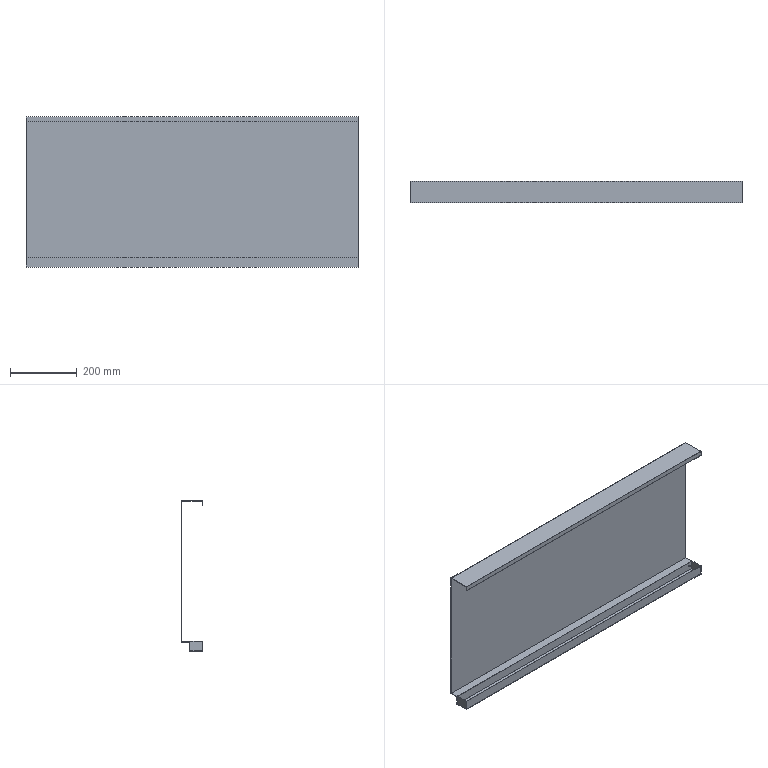Part | SolidWorks | features ICE 3, ExtruThin 1 | 3 solids | 34 faces | box 998 x 65 x 452 mm | volume 623910 mm3 | plane 30 | cylinder 4 | commonest cylinder face diameters 5.5 x4
STEP:
#1=CARTESIAN_POINT('',(0.,-26.,-401.));
#2=VERTEX_POINT('',#1);
#3=CARTESIAN_POINT('',(0.,-64.,-401.));
#4=VERTEX_POINT('',#3);
#5=CARTESIAN_POINT('',(0.,-64.,-401.));
#6=DIRECTION('',(0.,-1.,0.));
#7=VECTOR('',#6,1000.);
#8=LINE('',#5,#7);
#9=EDGE_CURVE('',#2,#4,#8,.T.);
#10=ORIENTED_EDGE('',*,*,#9,.F.);
#11=CARTESIAN_POINT('',(1.,-26.,-401.));
#12=VERTEX_POINT('',#11);
#13=CARTESIAN_POINT('',(1.,-26.,-401.));
#14=DIRECTION('',(-1.,0.,0.));
#15=VECTOR('',#14,1000.);
#16=LINE('',#13,#15);
#17=EDGE_CURVE('',#12,#2,#16,.T.);
#18=ORIENTED_EDGE('',*,*,#17,.F.);
#19=CARTESIAN_POINT('',(1.,-64.,-401.));
#20=VERTEX_POINT('',#19);
#21=CARTESIAN_POINT('',(1.,-64.,-401.));
#22=DIRECTION('',(0.,-1.,0.));
#23=VECTOR('',#22,1000.);
#24=LINE('',#21,#23);
#25=EDGE_CURVE('',#12,#20,#24,.T.);
#26=ORIENTED_EDGE('',*,*,#25,.T.);
#27=CARTESIAN_POINT('',(1.,-64.,-401.));
#28=DIRECTION('',(-1.,0.,0.));
#29=VECTOR('',#28,1000.);
#30=LINE('',#27,#29);
#31=EDGE_CURVE('',#20,#4,#30,.T.);
#32=ORIENTED_EDGE('',*,*,#31,.T.);
#33=EDGE_LOOP('',(#10,#18,#26,#32));
#34=FACE_OUTER_BOUND('',#33,.T.);
#35=CARTESIAN_POINT('',(1.,-64.,-401.));
#36=DIRECTION('',(0.,0.,-1.));
#37=DIRECTION('',(0.,1.,0.));
#38=AXIS2_PLACEMENT_3D('',#35,#36,#37);
#39=PLANE('',#38);
#40=ADVANCED_FACE('',(#34),#39,.T.);
#41=CARTESIAN_POINT('',(0.,-26.,-372.));
#42=VERTEX_POINT('',#41);
#43=CARTESIAN_POINT('',(0.,-26.,-401.));
#44=DIRECTION('',(0.,0.,-1.));
#45=VECTOR('',#44,1000.);
#46=LINE('',#43,#45);
#47=EDGE_CURVE('',#42,#2,#46,.T.);
#48=ORIENTED_EDGE('',*,*,#47,.F.);
#49=CARTESIAN_POINT('',(1.,-26.,-372.));
#50=VERTEX_POINT('',#49);
#51=CARTESIAN_POINT('',(1.,-26.,-372.));
#52=DIRECTION('',(-1.,0.,0.));
#53=VECTOR('',#52,1000.);
#54=LINE('',#51,#53);
#55=EDGE_CURVE('',#50,#42,#54,.T.);
#56=ORIENTED_EDGE('',*,*,#55,.F.);
#57=CARTESIAN_POINT('',(1.,-26.,-401.));
#58=DIRECTION('',(0.,0.,-1.));
#59=VECTOR('',#58,1000.);
#60=LINE('',#57,#59);
#61=EDGE_CURVE('',#50,#12,#60,.T.);
#62=ORIENTED_EDGE('',*,*,#61,.T.);
#63=ORIENTED_EDGE('',*,*,#17,.T.);
#64=EDGE_LOOP('',(#48,#56,#62,#63));
#65=FACE_OUTER_BOUND('',#64,.T.);
#66=CARTESIAN_POINT('',(1.,-26.,-401.));
#67=DIRECTION('',(0.,1.,0.));
#68=DIRECTION('',(0.,0.,1.));
#69=AXIS2_PLACEMENT_3D('',#66,#67,#68);
#70=PLANE('',#69);
#71=ADVANCED_FACE('',(#65),#70,.T.);
#72=CARTESIAN_POINT('',(0.,-64.,-372.));
#73=VERTEX_POINT('',#72);
#74=CARTESIAN_POINT('',(0.,-26.,-372.));
#75=DIRECTION('',(0.,1.,0.));
#76=VECTOR('',#75,1000.);
#77=LINE('',#74,#76);
#78=EDGE_CURVE('',#73,#42,#77,.T.);
#79=ORIENTED_EDGE('',*,*,#78,.F.);
#80=CARTESIAN_POINT('',(1.,-64.,-372.));
#81=VERTEX_POINT('',#80);
#82=CARTESIAN_POINT('',(1.,-64.,-372.));
#83=DIRECTION('',(-1.,0.,0.));
#84=VECTOR('',#83,1000.);
#85=LINE('',#82,#84);
#86=EDGE_CURVE('',#81,#73,#85,.T.);
#87=ORIENTED_EDGE('',*,*,#86,.F.);
#88=CARTESIAN_POINT('',(1.,-26.,-372.));
#89=DIRECTION('',(0.,1.,0.));
#90=VECTOR('',#89,1000.);
#91=LINE('',#88,#90);
#92=EDGE_CURVE('',#81,#50,#91,.T.);
#93=ORIENTED_EDGE('',*,*,#92,.T.);
#94=ORIENTED_EDGE('',*,*,#55,.T.);
#95=EDGE_LOOP('',(#79,#87,#93,#94));
#96=FACE_OUTER_BOUND('',#95,.T.);
#97=CARTESIAN_POINT('',(1.,-26.,-372.));
#98=DIRECTION('',(0.,0.,1.));
#99=DIRECTION('',(1.,0.,0.));
#100=AXIS2_PLACEMENT_3D('',#97,#98,#99);
#101=PLANE('',#100);
#102=ADVANCED_FACE('',(#96),#101,.T.);
#103=CARTESIAN_POINT('',(0.,-64.,-372.));
#104=DIRECTION('',(0.,0.,1.));
#105=VECTOR('',#104,1000.);
#106=LINE('',#103,#105);
#107=EDGE_CURVE('',#4,#73,#106,.T.);
#108=ORIENTED_EDGE('',*,*,#107,.F.);
#109=ORIENTED_EDGE('',*,*,#31,.F.);
#110=CARTESIAN_POINT('',(1.,-64.,-372.));
#111=DIRECTION('',(0.,0.,1.));
#112=VECTOR('',#111,1000.);
#113=LINE('',#110,#112);
#114=EDGE_CURVE('',#20,#81,#113,.T.);
#115=ORIENTED_EDGE('',*,*,#114,.T.);
#116=ORIENTED_EDGE('',*,*,#86,.T.);
#117=EDGE_LOOP('',(#108,#109,#115,#116));
#118=FACE_OUTER_BOUND('',#117,.T.);
#119=CARTESIAN_POINT('',(1.,-64.,-372.));
#120=DIRECTION('',(0.,-1.,0.));
#121=DIRECTION('',(0.,0.,-1.));
#122=AXIS2_PLACEMENT_3D('',#119,#120,#121);
#123=PLANE('',#122);
#124=ADVANCED_FACE('',(#118),#123,.T.);
#125=ORIENTED_EDGE('',*,*,#25,.F.);
#126=ORIENTED_EDGE('',*,*,#61,.F.);
#127=ORIENTED_EDGE('',*,*,#92,.F.);
#128=ORIENTED_EDGE('',*,*,#114,.F.);
#129=EDGE_LOOP('',(#125,#126,#127,#128));
#130=FACE_OUTER_BOUND('',#129,.T.);
#131=CARTESIAN_POINT('',(1.,-26.,-401.));
#132=DIRECTION('',(1.,0.,0.));
#133=DIRECTION('',(0.,0.,-1.));
#134=AXIS2_PLACEMENT_3D('',#131,#132,#133);
#135=PLANE('',#134);
#136=ADVANCED_FACE('',(#130),#135,.T.);
#137=ORIENTED_EDGE('',*,*,#9,.T.);
#138=ORIENTED_EDGE('',*,*,#107,.T.);
#139=ORIENTED_EDGE('',*,*,#78,.T.);
#140=ORIENTED_EDGE('',*,*,#47,.T.);
#141=EDGE_LOOP('',(#137,#138,#139,#140));
#142=FACE_OUTER_BOUND('',#141,.T.);
#143=CARTESIAN_POINT('',(0.,-26.,-401.));
#144=DIRECTION('',(1.,0.,0.));
#145=DIRECTION('',(0.,0.,-1.));
#146=AXIS2_PLACEMENT_3D('',#143,#144,#145);
#147=PLANE('',#146);
#148=ADVANCED_FACE('',(#142),#147,.F.);
#149=CLOSED_SHELL('',(#40,#71,#102,#124,#136,#148));
#150=MANIFOLD_SOLID_BREP('',#149);
#151=CARTESIAN_POINT('',(998.,-26.,-372.));
#152=VERTEX_POINT('',#151);
#153=CARTESIAN_POINT('',(998.,-64.,-372.));
#154=VERTEX_POINT('',#153);
#155=CARTESIAN_POINT('',(998.,-26.,-372.));
#156=DIRECTION('',(0.,-1.,0.));
#157=VECTOR('',#156,1000.);
#158=LINE('',#155,#157);
#159=EDGE_CURVE('',#152,#154,#158,.T.);
#160=ORIENTED_EDGE('',*,*,#159,.F.);
#161=CARTESIAN_POINT('',(997.,-26.,-372.));
#162=VERTEX_POINT('',#161);
#163=CARTESIAN_POINT('',(997.,-26.,-372.));
#164=DIRECTION('',(1.,0.,0.));
#165=VECTOR('',#164,1000.);
#166=LINE('',#163,#165);
#167=EDGE_CURVE('',#162,#152,#166,.T.);
#168=ORIENTED_EDGE('',*,*,#167,.F.);
#169=CARTESIAN_POINT('',(997.,-64.,-372.));
#170=VERTEX_POINT('',#169);
#171=CARTESIAN_POINT('',(997.,-26.,-372.));
#172=DIRECTION('',(0.,-1.,0.));
#173=VECTOR('',#172,1000.);
#174=LINE('',#171,#173);
#175=EDGE_CURVE('',#162,#170,#174,.T.);
#176=ORIENTED_EDGE('',*,*,#175,.T.);
#177=CARTESIAN_POINT('',(997.,-64.,-372.));
#178=DIRECTION('',(1.,0.,0.));
#179=VECTOR('',#178,1000.);
#180=LINE('',#177,#179);
#181=EDGE_CURVE('',#170,#154,#180,.T.);
#182=ORIENTED_EDGE('',*,*,#181,.T.);
#183=EDGE_LOOP('',(#160,#168,#176,#182));
#184=FACE_OUTER_BOUND('',#183,.T.);
#185=CARTESIAN_POINT('',(997.,-26.,-372.));
#186=DIRECTION('',(0.,0.,1.));
#187=DIRECTION('',(1.,0.,0.));
#188=AXIS2_PLACEMENT_3D('',#185,#186,#187);
#189=PLANE('',#188);
#190=ADVANCED_FACE('',(#184),#189,.T.);
#191=CARTESIAN_POINT('',(998.,-26.,-401.));
#192=VERTEX_POINT('',#191);
#193=CARTESIAN_POINT('',(998.,-26.,-401.));
#194=DIRECTION('',(0.,0.,1.));
#195=VECTOR('',#194,1000.);
#196=LINE('',#193,#195);
#197=EDGE_CURVE('',#192,#152,#196,.T.);
#198=ORIENTED_EDGE('',*,*,#197,.F.);
#199=CARTESIAN_POINT('',(997.,-26.,-401.));
#200=VERTEX_POINT('',#199);
#201=CARTESIAN_POINT('',(997.,-26.,-401.));
#202=DIRECTION('',(1.,0.,0.));
#203=VECTOR('',#202,1000.);
#204=LINE('',#201,#203);
#205=EDGE_CURVE('',#200,#192,#204,.T.);
#206=ORIENTED_EDGE('',*,*,#205,.F.);
#207=CARTESIAN_POINT('',(997.,-26.,-401.));
#208=DIRECTION('',(0.,0.,1.));
#209=VECTOR('',#208,1000.);
#210=LINE('',#207,#209);
#211=EDGE_CURVE('',#200,#162,#210,.T.);
#212=ORIENTED_EDGE('',*,*,#211,.T.);
#213=ORIENTED_EDGE('',*,*,#167,.T.);
#214=EDGE_LOOP('',(#198,#206,#212,#213));
#215=FACE_OUTER_BOUND('',#214,.T.);
#216=CARTESIAN_POINT('',(997.,-26.,-401.));
#217=DIRECTION('',(0.,1.,0.));
#218=DIRECTION('',(0.,0.,1.));
#219=AXIS2_PLACEMENT_3D('',#216,#217,#218);
#220=PLANE('',#219);
#221=ADVANCED_FACE('',(#215),#220,.T.);
#222=CARTESIAN_POINT('',(998.,-64.,-401.));
#223=VERTEX_POINT('',#222);
#224=CARTESIAN_POINT('',(998.,-64.,-401.));
#225=DIRECTION('',(0.,1.,0.));
#226=VECTOR('',#225,1000.);
#227=LINE('',#224,#226);
#228=EDGE_CURVE('',#223,#192,#227,.T.);
#229=ORIENTED_EDGE('',*,*,#228,.F.);
#230=CARTESIAN_POINT('',(997.,-64.,-401.));
#231=VERTEX_POINT('',#230);
#232=CARTESIAN_POINT('',(997.,-64.,-401.));
#233=DIRECTION('',(1.,0.,0.));
#234=VECTOR('',#233,1000.);
#235=LINE('',#232,#234);
#236=EDGE_CURVE('',#231,#223,#235,.T.);
#237=ORIENTED_EDGE('',*,*,#236,.F.);
#238=CARTESIAN_POINT('',(997.,-64.,-401.));
#239=DIRECTION('',(0.,1.,0.));
#240=VECTOR('',#239,1000.);
#241=LINE('',#238,#240);
#242=EDGE_CURVE('',#231,#200,#241,.T.);
#243=ORIENTED_EDGE('',*,*,#242,.T.);
#244=ORIENTED_EDGE('',*,*,#205,.T.);
#245=EDGE_LOOP('',(#229,#237,#243,#244));
#246=FACE_OUTER_BOUND('',#245,.T.);
#247=CARTESIAN_POINT('',(997.,-64.,-401.));
#248=DIRECTION('',(0.,0.,-1.));
#249=DIRECTION('',(0.,1.,0.));
#250=AXIS2_PLACEMENT_3D('',#247,#248,#249);
#251=PLANE('',#250);
#252=ADVANCED_FACE('',(#246),#251,.T.);
#253=CARTESIAN_POINT('',(998.,-64.,-372.));
#254=DIRECTION('',(0.,0.,-1.));
#255=VECTOR('',#254,1000.);
#256=LINE('',#253,#255);
#257=EDGE_CURVE('',#154,#223,#256,.T.);
#258=ORIENTED_EDGE('',*,*,#257,.F.);
#259=ORIENTED_EDGE('',*,*,#181,.F.);
#260=CARTESIAN_POINT('',(997.,-64.,-372.));
#261=DIRECTION('',(0.,0.,-1.));
#262=VECTOR('',#261,1000.);
#263=LINE('',#260,#262);
#264=EDGE_CURVE('',#170,#231,#263,.T.);
#265=ORIENTED_EDGE('',*,*,#264,.T.);
#266=ORIENTED_EDGE('',*,*,#236,.T.);
#267=EDGE_LOOP('',(#258,#259,#265,#266));
#268=FACE_OUTER_BOUND('',#267,.T.);
#269=CARTESIAN_POINT('',(997.,-64.,-372.));
#270=DIRECTION('',(0.,-1.,0.));
#271=DIRECTION('',(0.,0.,-1.));
#272=AXIS2_PLACEMENT_3D('',#269,#270,#271);
#273=PLANE('',#272);
#274=ADVANCED_FACE('',(#268),#273,.T.);
#275=ORIENTED_EDGE('',*,*,#175,.F.);
#276=ORIENTED_EDGE('',*,*,#211,.F.);
#277=ORIENTED_EDGE('',*,*,#242,.F.);
#278=ORIENTED_EDGE('',*,*,#264,.F.);
#279=EDGE_LOOP('',(#275,#276,#277,#278));
#280=FACE_OUTER_BOUND('',#279,.T.);
#281=CARTESIAN_POINT('',(997.,-64.,-372.));
#282=DIRECTION('',(1.,0.,0.));
#283=DIRECTION('',(0.,0.,-1.));
#284=AXIS2_PLACEMENT_3D('',#281,#282,#283);
#285=PLANE('',#284);
#286=ADVANCED_FACE('',(#280),#285,.F.);
#287=ORIENTED_EDGE('',*,*,#159,.T.);
#288=ORIENTED_EDGE('',*,*,#257,.T.);
#289=ORIENTED_EDGE('',*,*,#228,.T.);
#290=ORIENTED_EDGE('',*,*,#197,.T.);
#291=EDGE_LOOP('',(#287,#288,#289,#290));
#292=FACE_OUTER_BOUND('',#291,.T.);
#293=CARTESIAN_POINT('',(998.,-64.,-372.));
#294=DIRECTION('',(1.,0.,0.));
#295=DIRECTION('',(0.,0.,-1.));
#296=AXIS2_PLACEMENT_3D('',#293,#294,#295);
#297=PLANE('',#296);
#298=ADVANCED_FACE('',(#292),#297,.T.);
#299=CLOSED_SHELL('',(#190,#221,#252,#274,#286,#298));
#300=MANIFOLD_SOLID_BREP('',#299);
#301=CARTESIAN_POINT('',(988.,-26.,-384.25));
#302=VERTEX_POINT('',#301);
#303=CARTESIAN_POINT('',(988.,-26.,-389.75));
#304=VERTEX_POINT('',#303);
#305=CARTESIAN_POINT('',(988.,-26.,-387.));
#306=DIRECTION('',(0.,-1.,0.));
#307=DIRECTION('',(0.,0.,-1.));
#308=AXIS2_PLACEMENT_3D('',#305,#306,#307);
#309=CIRCLE('',#308,2.75);
#310=EDGE_CURVE('',#302,#304,#309,.T.);
#311=ORIENTED_EDGE('',*,*,#310,.T.);
#312=CARTESIAN_POINT('',(988.,-25.,-389.75));
#313=VERTEX_POINT('',#312);
#314=CARTESIAN_POINT('',(988.,-35.,-389.75));
#315=DIRECTION('',(0.,1.,0.));
#316=VECTOR('',#315,1000.);
#317=LINE('',#314,#316);
#318=EDGE_CURVE('',#304,#313,#317,.T.);
#319=ORIENTED_EDGE('',*,*,#318,.T.);
#320=CARTESIAN_POINT('',(988.,-25.,-384.25));
#321=VERTEX_POINT('',#320);
#322=CARTESIAN_POINT('',(988.,-25.,-387.));
#323=DIRECTION('',(0.,1.,0.));
#324=DIRECTION('',(0.,0.,1.));
#325=AXIS2_PLACEMENT_3D('',#322,#323,#324);
#326=CIRCLE('',#325,2.75);
#327=EDGE_CURVE('',#313,#321,#326,.T.);
#328=ORIENTED_EDGE('',*,*,#327,.T.);
#329=CARTESIAN_POINT('',(988.,-35.,-384.25));
#330=DIRECTION('',(0.,1.,0.));
#331=VECTOR('',#330,1000.);
#332=LINE('',#329,#331);
#333=EDGE_CURVE('',#302,#321,#332,.T.);
#334=ORIENTED_EDGE('',*,*,#333,.F.);
#335=EDGE_LOOP('',(#311,#319,#328,#334));
#336=FACE_OUTER_BOUND('',#335,.T.);
#337=CARTESIAN_POINT('',(988.,-35.,-387.));
#338=DIRECTION('',(0.,1.,0.));
#339=DIRECTION('',(0.,0.,1.));
#340=AXIS2_PLACEMENT_3D('',#337,#338,#339);
#341=CYLINDRICAL_SURFACE('',#340,2.75);
#342=ADVANCED_FACE('',(#336),#341,.F.);
#343=CARTESIAN_POINT('',(13.,-26.,-386.25));
#344=VERTEX_POINT('',#343);
#345=CARTESIAN_POINT('',(13.,-26.,-391.75));
#346=VERTEX_POINT('',#345);
#347=CARTESIAN_POINT('',(13.,-26.,-389.));
#348=DIRECTION('',(0.,-1.,0.));
#349=DIRECTION('',(0.,0.,-1.));
#350=AXIS2_PLACEMENT_3D('',#347,#348,#349);
#351=CIRCLE('',#350,2.75);
#352=EDGE_CURVE('',#344,#346,#351,.T.);
#353=ORIENTED_EDGE('',*,*,#352,.T.);
#354=CARTESIAN_POINT('',(13.,-25.,-391.75));
#355=VERTEX_POINT('',#354);
#356=CARTESIAN_POINT('',(13.,-35.,-391.75));
#357=DIRECTION('',(0.,1.,0.));
#358=VECTOR('',#357,1000.);
#359=LINE('',#356,#358);
#360=EDGE_CURVE('',#346,#355,#359,.T.);
#361=ORIENTED_EDGE('',*,*,#360,.T.);
#362=CARTESIAN_POINT('',(13.,-25.,-386.25));
#363=VERTEX_POINT('',#362);
#364=CARTESIAN_POINT('',(13.,-25.,-389.));
#365=DIRECTION('',(0.,1.,0.));
#366=DIRECTION('',(0.,0.,1.));
#367=AXIS2_PLACEMENT_3D('',#364,#365,#366);
#368=CIRCLE('',#367,2.75);
#369=EDGE_CURVE('',#355,#363,#368,.T.);
#370=ORIENTED_EDGE('',*,*,#369,.T.);
#371=CARTESIAN_POINT('',(13.,-35.,-386.25));
#372=DIRECTION('',(0.,1.,0.));
#373=VECTOR('',#372,1000.);
#374=LINE('',#371,#373);
#375=EDGE_CURVE('',#344,#363,#374,.T.);
#376=ORIENTED_EDGE('',*,*,#375,.F.);
#377=EDGE_LOOP('',(#353,#361,#370,#376));
#378=FACE_OUTER_BOUND('',#377,.T.);
#379=CARTESIAN_POINT('',(13.,-35.,-389.));
#380=DIRECTION('',(0.,1.,0.));
#381=DIRECTION('',(0.,0.,1.));
#382=AXIS2_PLACEMENT_3D('',#379,#380,#381);
#383=CYLINDRICAL_SURFACE('',#382,2.75);
#384=ADVANCED_FACE('',(#378),#383,.F.);
#385=CARTESIAN_POINT('',(0.,-65.,50.));
#386=VERTEX_POINT('',#385);
#387=CARTESIAN_POINT('',(0.,-65.,35.));
#388=VERTEX_POINT('',#387);
#389=CARTESIAN_POINT('',(0.,-65.,50.));
#390=DIRECTION('',(0.,0.,-1.));
#391=VECTOR('',#390,1000.);
#392=LINE('',#389,#391);
#393=EDGE_CURVE('',#386,#388,#392,.T.);
#394=ORIENTED_EDGE('',*,*,#393,.T.);
#395=CARTESIAN_POINT('',(998.,-65.,35.));
#396=VERTEX_POINT('',#395);
#397=CARTESIAN_POINT('',(998.,-65.,35.));
#398=DIRECTION('',(-1.,0.,0.));
#399=VECTOR('',#398,1000.);
#400=LINE('',#397,#399);
#401=EDGE_CURVE('',#396,#388,#400,.T.);
#402=ORIENTED_EDGE('',*,*,#401,.F.);
#403=CARTESIAN_POINT('',(998.,-65.,50.));
#404=VERTEX_POINT('',#403);
#405=CARTESIAN_POINT('',(998.,-65.,50.));
#406=DIRECTION('',(0.,0.,-1.));
#407=VECTOR('',#406,1000.);
#408=LINE('',#405,#407);
#409=EDGE_CURVE('',#404,#396,#408,.T.);
#410=ORIENTED_EDGE('',*,*,#409,.F.);
#411=CARTESIAN_POINT('',(998.,-65.,50.));
#412=DIRECTION('',(-1.,0.,0.));
#413=VECTOR('',#412,1000.);
#414=LINE('',#411,#413);
#415=EDGE_CURVE('',#404,#386,#414,.T.);
#416=ORIENTED_EDGE('',*,*,#415,.T.);
#417=EDGE_LOOP('',(#394,#402,#410,#416));
#418=FACE_OUTER_BOUND('',#417,.T.);
#419=CARTESIAN_POINT('',(998.,-65.,50.));
#420=DIRECTION('',(0.,1.,0.));
#421=DIRECTION('',(0.,0.,1.));
#422=AXIS2_PLACEMENT_3D('',#419,#420,#421);
#423=PLANE('',#422);
#424=ADVANCED_FACE('',(#418),#423,.F.);
#425=CARTESIAN_POINT('',(0.,-64.,35.));
#426=VERTEX_POINT('',#425);
#427=CARTESIAN_POINT('',(0.,-64.,35.));
#428=DIRECTION('',(0.,-1.,0.));
#429=VECTOR('',#428,1000.);
#430=LINE('',#427,#429);
#431=EDGE_CURVE('',#426,#388,#430,.T.);
#432=ORIENTED_EDGE('',*,*,#431,.F.);
#433=CARTESIAN_POINT('',(998.,-64.,35.));
#434=VERTEX_POINT('',#433);
#435=CARTESIAN_POINT('',(998.,-64.,35.));
#436=DIRECTION('',(-1.,0.,0.));
#437=VECTOR('',#436,1000.);
#438=LINE('',#435,#437);
#439=EDGE_CURVE('',#434,#426,#438,.T.);
#440=ORIENTED_EDGE('',*,*,#439,.F.);
#441=CARTESIAN_POINT('',(998.,-64.,35.));
#442=DIRECTION('',(0.,-1.,0.));
#443=VECTOR('',#442,1000.);
#444=LINE('',#441,#443);
#445=EDGE_CURVE('',#434,#396,#444,.T.);
#446=ORIENTED_EDGE('',*,*,#445,.T.);
#447=ORIENTED_EDGE('',*,*,#401,.T.);
#448=EDGE_LOOP('',(#432,#440,#446,#447));
#449=FACE_OUTER_BOUND('',#448,.T.);
#450=CARTESIAN_POINT('',(998.,-64.,35.));
#451=DIRECTION('',(0.,0.,-1.));
#452=DIRECTION('',(-1.,0.,0.));
#453=AXIS2_PLACEMENT_3D('',#450,#451,#452);
#454=PLANE('',#453);
#455=ADVANCED_FACE('',(#449),#454,.T.);
#456=CARTESIAN_POINT('',(0.,-64.,49.));
#457=VERTEX_POINT('',#456);
#458=CARTESIAN_POINT('',(0.,-64.,50.));
#459=DIRECTION('',(0.,0.,-1.));
#460=VECTOR('',#459,1000.);
#461=LINE('',#458,#460);
#462=EDGE_CURVE('',#457,#426,#461,.T.);
#463=ORIENTED_EDGE('',*,*,#462,.F.);
#464=CARTESIAN_POINT('',(998.,-64.,49.));
#465=VERTEX_POINT('',#464);
#466=CARTESIAN_POINT('',(998.,-64.,49.));
#467=DIRECTION('',(-1.,0.,0.));
#468=VECTOR('',#467,1000.);
#469=LINE('',#466,#468);
#470=EDGE_CURVE('',#465,#457,#469,.T.);
#471=ORIENTED_EDGE('',*,*,#470,.F.);
#472=CARTESIAN_POINT('',(998.,-64.,50.));
#473=DIRECTION('',(0.,0.,-1.));
#474=VECTOR('',#473,1000.);
#475=LINE('',#472,#474);
#476=EDGE_CURVE('',#465,#434,#475,.T.);
#477=ORIENTED_EDGE('',*,*,#476,.T.);
#478=ORIENTED_EDGE('',*,*,#439,.T.);
#479=EDGE_LOOP('',(#463,#471,#477,#478));
#480=FACE_OUTER_BOUND('',#479,.T.);
#481=CARTESIAN_POINT('',(998.,-64.,50.));
#482=DIRECTION('',(0.,1.,0.));
#483=DIRECTION('',(0.,0.,1.));
#484=AXIS2_PLACEMENT_3D('',#481,#482,#483);
#485=PLANE('',#484);
#486=ADVANCED_FACE('',(#480),#485,.T.);
#487=CARTESIAN_POINT('',(0.,-1.,49.));
#488=VERTEX_POINT('',#487);
#489=CARTESIAN_POINT('',(0.,0.,49.));
#490=DIRECTION('',(0.,-1.,0.));
#491=VECTOR('',#490,1000.);
#492=LINE('',#489,#491);
#493=EDGE_CURVE('',#488,#457,#492,.T.);
#494=ORIENTED_EDGE('',*,*,#493,.F.);
#495=CARTESIAN_POINT('',(998.,-1.,49.));
#496=VERTEX_POINT('',#495);
#497=CARTESIAN_POINT('',(998.,-1.,49.));
#498=DIRECTION('',(-1.,0.,0.));
#499=VECTOR('',#498,1000.);
#500=LINE('',#497,#499);
#501=EDGE_CURVE('',#496,#488,#500,.T.);
#502=ORIENTED_EDGE('',*,*,#501,.F.);
#503=CARTESIAN_POINT('',(998.,0.,49.));
#504=DIRECTION('',(0.,-1.,0.));
#505=VECTOR('',#504,1000.);
#506=LINE('',#503,#505);
#507=EDGE_CURVE('',#496,#465,#506,.T.);
#508=ORIENTED_EDGE('',*,*,#507,.T.);
#509=ORIENTED_EDGE('',*,*,#470,.T.);
#510=EDGE_LOOP('',(#494,#502,#508,#509));
#511=FACE_OUTER_BOUND('',#510,.T.);
#512=CARTESIAN_POINT('',(998.,0.,49.));
#513=DIRECTION('',(0.,0.,-1.));
#514=DIRECTION('',(0.,1.,0.));
#515=AXIS2_PLACEMENT_3D('',#512,#513,#514);
#516=PLANE('',#515);
#517=ADVANCED_FACE('',(#511),#516,.T.);
#518=CARTESIAN_POINT('',(0.,-1.,-374.));
#519=VERTEX_POINT('',#518);
#520=CARTESIAN_POINT('',(0.,-1.,0.));
#521=DIRECTION('',(0.,0.,1.));
#522=VECTOR('',#521,1000.);
#523=LINE('',#520,#522);
#524=EDGE_CURVE('',#519,#488,#523,.T.);
#525=ORIENTED_EDGE('',*,*,#524,.F.);
#526=CARTESIAN_POINT('',(998.,-1.,-374.));
#527=VERTEX_POINT('',#526);
#528=CARTESIAN_POINT('',(998.,-1.,-374.));
#529=DIRECTION('',(-1.,0.,0.));
#530=VECTOR('',#529,1000.);
#531=LINE('',#528,#530);
#532=EDGE_CURVE('',#527,#519,#531,.T.);
#533=ORIENTED_EDGE('',*,*,#532,.F.);
#534=CARTESIAN_POINT('',(998.,-1.,0.));
#535=DIRECTION('',(0.,0.,1.));
#536=VECTOR('',#535,1000.);
#537=LINE('',#534,#536);
#538=EDGE_CURVE('',#527,#496,#537,.T.);
#539=ORIENTED_EDGE('',*,*,#538,.T.);
#540=ORIENTED_EDGE('',*,*,#501,.T.);
#541=EDGE_LOOP('',(#525,#533,#539,#540));
#542=FACE_OUTER_BOUND('',#541,.T.);
#543=CARTESIAN_POINT('',(998.,-1.,0.));
#544=DIRECTION('',(0.,-1.,0.));
#545=DIRECTION('',(0.,0.,-1.));
#546=AXIS2_PLACEMENT_3D('',#543,#544,#545);
#547=PLANE('',#546);
#548=ADVANCED_FACE('',(#542),#547,.T.);
#549=CARTESIAN_POINT('',(0.,-26.,-374.));
#550=VERTEX_POINT('',#549);
#551=CARTESIAN_POINT('',(0.,0.,-374.));
#552=DIRECTION('',(0.,1.,0.));
#553=VECTOR('',#552,1000.);
#554=LINE('',#551,#553);
#555=EDGE_CURVE('',#550,#519,#554,.T.);
#556=ORIENTED_EDGE('',*,*,#555,.F.);
#557=CARTESIAN_POINT('',(998.,-26.,-374.));
#558=VERTEX_POINT('',#557);
#559=CARTESIAN_POINT('',(998.,-26.,-374.));
#560=DIRECTION('',(-1.,0.,0.));
#561=VECTOR('',#560,1000.);
#562=LINE('',#559,#561);
#563=EDGE_CURVE('',#558,#550,#562,.T.);
#564=ORIENTED_EDGE('',*,*,#563,.F.);
#565=CARTESIAN_POINT('',(998.,0.,-374.));
#566=DIRECTION('',(0.,1.,0.));
#567=VECTOR('',#566,1000.);
#568=LINE('',#565,#567);
#569=EDGE_CURVE('',#558,#527,#568,.T.);
#570=ORIENTED_EDGE('',*,*,#569,.T.);
#571=ORIENTED_EDGE('',*,*,#532,.T.);
#572=EDGE_LOOP('',(#556,#564,#570,#571));
#573=FACE_OUTER_BOUND('',#572,.T.);
#574=CARTESIAN_POINT('',(998.,0.,-374.));
#575=DIRECTION('',(0.,0.,1.));
#576=DIRECTION('',(1.,0.,0.));
#577=AXIS2_PLACEMENT_3D('',#574,#575,#576);
#578=PLANE('',#577);
#579=ADVANCED_FACE('',(#573),#578,.T.);
#580=ORIENTED_EDGE('',*,*,#310,.F.);
#581=CARTESIAN_POINT('',(988.,-26.,-387.));
#582=DIRECTION('',(0.,-1.,0.));
#583=DIRECTION('',(0.,0.,-1.));
#584=AXIS2_PLACEMENT_3D('',#581,#582,#583);
#585=CIRCLE('',#584,2.75);
#586=EDGE_CURVE('',#304,#302,#585,.T.);
#587=ORIENTED_EDGE('',*,*,#586,.F.);
#588=EDGE_LOOP('',(#580,#587));
#589=FACE_BOUND('',#588,.T.);
#590=ORIENTED_EDGE('',*,*,#352,.F.);
#591=CARTESIAN_POINT('',(13.,-26.,-389.));
#592=DIRECTION('',(0.,-1.,0.));
#593=DIRECTION('',(0.,0.,-1.));
#594=AXIS2_PLACEMENT_3D('',#591,#592,#593);
#595=CIRCLE('',#594,2.75);
#596=EDGE_CURVE('',#346,#344,#595,.T.);
#597=ORIENTED_EDGE('',*,*,#596,.F.);
#598=EDGE_LOOP('',(#590,#597));
#599=FACE_BOUND('',#598,.T.);
#600=CARTESIAN_POINT('',(0.,-26.,-401.));
#601=VERTEX_POINT('',#600);
#602=CARTESIAN_POINT('',(0.,-26.,-375.));
#603=DIRECTION('',(0.,0.,1.));
#604=VECTOR('',#603,1000.);
#605=LINE('',#602,#604);
#606=EDGE_CURVE('',#601,#550,#605,.T.);
#607=ORIENTED_EDGE('',*,*,#606,.F.);
#608=CARTESIAN_POINT('',(998.,-26.,-401.));
#609=VERTEX_POINT('',#608);
#610=CARTESIAN_POINT('',(998.,-26.,-401.));
#611=DIRECTION('',(-1.,0.,0.));
#612=VECTOR('',#611,1000.);
#613=LINE('',#610,#612);
#614=EDGE_CURVE('',#609,#601,#613,.T.);
#615=ORIENTED_EDGE('',*,*,#614,.F.);
#616=CARTESIAN_POINT('',(998.,-26.,-375.));
#617=DIRECTION('',(0.,0.,1.));
#618=VECTOR('',#617,1000.);
#619=LINE('',#616,#618);
#620=EDGE_CURVE('',#609,#558,#619,.T.);
#621=ORIENTED_EDGE('',*,*,#620,.T.);
#622=ORIENTED_EDGE('',*,*,#563,.T.);
#623=EDGE_LOOP('',(#607,#615,#621,#622));
#624=FACE_OUTER_BOUND('',#623,.T.);
#625=CARTESIAN_POINT('',(998.,-26.,-375.));
#626=DIRECTION('',(0.,-1.,0.));
#627=DIRECTION('',(0.,0.,-1.));
#628=AXIS2_PLACEMENT_3D('',#625,#626,#627);
#629=PLANE('',#628);
#630=ADVANCED_FACE('',(#589,#599,#624),#629,.T.);
#631=CARTESIAN_POINT('',(0.,-64.,-401.));
#632=VERTEX_POINT('',#631);
#633=CARTESIAN_POINT('',(0.,-25.,-401.));
#634=DIRECTION('',(0.,1.,0.));
#635=VECTOR('',#634,1000.);
#636=LINE('',#633,#635);
#637=EDGE_CURVE('',#632,#601,#636,.T.);
#638=ORIENTED_EDGE('',*,*,#637,.F.);
#639=CARTESIAN_POINT('',(998.,-64.,-401.));
#640=VERTEX_POINT('',#639);
#641=CARTESIAN_POINT('',(998.,-64.,-401.));
#642=DIRECTION('',(-1.,0.,0.));
#643=VECTOR('',#642,1000.);
#644=LINE('',#641,#643);
#645=EDGE_CURVE('',#640,#632,#644,.T.);
#646=ORIENTED_EDGE('',*,*,#645,.F.);
#647=CARTESIAN_POINT('',(998.,-25.,-401.));
#648=DIRECTION('',(0.,1.,0.));
#649=VECTOR('',#648,1000.);
#650=LINE('',#647,#649);
#651=EDGE_CURVE('',#640,#609,#650,.T.);
#652=ORIENTED_EDGE('',*,*,#651,.T.);
#653=ORIENTED_EDGE('',*,*,#614,.T.);
#654=EDGE_LOOP('',(#638,#646,#652,#653));
#655=FACE_OUTER_BOUND('',#654,.T.);
#656=CARTESIAN_POINT('',(998.,-25.,-401.));
#657=DIRECTION('',(0.,0.,1.));
#658=DIRECTION('',(0.,-1.,0.));
#659=AXIS2_PLACEMENT_3D('',#656,#657,#658);
#660=PLANE('',#659);
#661=ADVANCED_FACE('',(#655),#660,.T.);
#662=CARTESIAN_POINT('',(0.,-64.,-372.));
#663=VERTEX_POINT('',#662);
#664=CARTESIAN_POINT('',(0.,-64.,-402.));
#665=DIRECTION('',(0.,0.,-1.));
#666=VECTOR('',#665,1000.);
#667=LINE('',#664,#666);
#668=EDGE_CURVE('',#663,#632,#667,.T.);
#669=ORIENTED_EDGE('',*,*,#668,.F.);
#670=CARTESIAN_POINT('',(998.,-64.,-372.));
#671=VERTEX_POINT('',#670);
#672=CARTESIAN_POINT('',(998.,-64.,-372.));
#673=DIRECTION('',(-1.,0.,0.));
#674=VECTOR('',#673,1000.);
#675=LINE('',#672,#674);
#676=EDGE_CURVE('',#671,#663,#675,.T.);
#677=ORIENTED_EDGE('',*,*,#676,.F.);
#678=CARTESIAN_POINT('',(998.,-64.,-402.));
#679=DIRECTION('',(0.,0.,-1.));
#680=VECTOR('',#679,1000.);
#681=LINE('',#678,#680);
#682=EDGE_CURVE('',#671,#640,#681,.T.);
#683=ORIENTED_EDGE('',*,*,#682,.T.);
#684=ORIENTED_EDGE('',*,*,#645,.T.);
#685=EDGE_LOOP('',(#669,#677,#683,#684));
#686=FACE_OUTER_BOUND('',#685,.T.);
#687=CARTESIAN_POINT('',(998.,-64.,-402.));
#688=DIRECTION('',(0.,1.,0.));
#689=DIRECTION('',(0.,0.,1.));
#690=AXIS2_PLACEMENT_3D('',#687,#688,#689);
#691=PLANE('',#690);
#692=ADVANCED_FACE('',(#686),#691,.T.);
#693=CARTESIAN_POINT('',(0.,-65.,-372.));
#694=VERTEX_POINT('',#693);
#695=CARTESIAN_POINT('',(0.,-65.,-372.));
#696=DIRECTION('',(0.,1.,0.));
#697=VECTOR('',#696,1000.);
#698=LINE('',#695,#697);
#699=EDGE_CURVE('',#694,#663,#698,.T.);
#700=ORIENTED_EDGE('',*,*,#699,.F.);
#701=CARTESIAN_POINT('',(998.,-65.,-372.));
#702=VERTEX_POINT('',#701);
#703=CARTESIAN_POINT('',(998.,-65.,-372.));
#704=DIRECTION('',(-1.,0.,0.));
#705=VECTOR('',#704,1000.);
#706=LINE('',#703,#705);
#707=EDGE_CURVE('',#702,#694,#706,.T.);
#708=ORIENTED_EDGE('',*,*,#707,.F.);
#709=CARTESIAN_POINT('',(998.,-65.,-372.));
#710=DIRECTION('',(0.,1.,0.));
#711=VECTOR('',#710,1000.);
#712=LINE('',#709,#711);
#713=EDGE_CURVE('',#702,#671,#712,.T.);
#714=ORIENTED_EDGE('',*,*,#713,.T.);
#715=ORIENTED_EDGE('',*,*,#676,.T.);
#716=EDGE_LOOP('',(#700,#708,#714,#715));
#717=FACE_OUTER_BOUND('',#716,.T.);
#718=CARTESIAN_POINT('',(998.,-65.,-372.));
#719=DIRECTION('',(0.,0.,1.));
#720=DIRECTION('',(1.,0.,0.));
#721=AXIS2_PLACEMENT_3D('',#718,#719,#720);
#722=PLANE('',#721);
#723=ADVANCED_FACE('',(#717),#722,.T.);
#724=CARTESIAN_POINT('',(0.,-65.,-402.));
#725=VERTEX_POINT('',#724);
#726=CARTESIAN_POINT('',(0.,-65.,-402.));
#727=DIRECTION('',(0.,0.,-1.));
#728=VECTOR('',#727,1000.);
#729=LINE('',#726,#728);
#730=EDGE_CURVE('',#694,#725,#729,.T.);
#731=ORIENTED_EDGE('',*,*,#730,.T.);
#732=CARTESIAN_POINT('',(998.,-65.,-402.));
#733=VERTEX_POINT('',#732);
#734=CARTESIAN_POINT('',(998.,-65.,-402.));
#735=DIRECTION('',(-1.,0.,0.));
#736=VECTOR('',#735,1000.);
#737=LINE('',#734,#736);
#738=EDGE_CURVE('',#733,#725,#737,.T.);
#739=ORIENTED_EDGE('',*,*,#738,.F.);
#740=CARTESIAN_POINT('',(998.,-65.,-402.));
#741=DIRECTION('',(0.,0.,-1.));
#742=VECTOR('',#741,1000.);
#743=LINE('',#740,#742);
#744=EDGE_CURVE('',#702,#733,#743,.T.);
#745=ORIENTED_EDGE('',*,*,#744,.F.);
#746=ORIENTED_EDGE('',*,*,#707,.T.);
#747=EDGE_LOOP('',(#731,#739,#745,#746));
#748=FACE_OUTER_BOUND('',#747,.T.);
#749=CARTESIAN_POINT('',(998.,-65.,-402.));
#750=DIRECTION('',(0.,1.,0.));
#751=DIRECTION('',(0.,0.,1.));
#752=AXIS2_PLACEMENT_3D('',#749,#750,#751);
#753=PLANE('',#752);
#754=ADVANCED_FACE('',(#748),#753,.F.);
#755=CARTESIAN_POINT('',(0.,-25.,-402.));
#756=VERTEX_POINT('',#755);
#757=CARTESIAN_POINT('',(0.,-25.,-402.));
#758=DIRECTION('',(0.,1.,0.));
#759=VECTOR('',#758,1000.);
#760=LINE('',#757,#759);
#761=EDGE_CURVE('',#725,#756,#760,.T.);
#762=ORIENTED_EDGE('',*,*,#761,.T.);
#763=CARTESIAN_POINT('',(998.,-25.,-402.));
#764=VERTEX_POINT('',#763);
#765=CARTESIAN_POINT('',(998.,-25.,-402.));
#766=DIRECTION('',(-1.,0.,0.));
#767=VECTOR('',#766,1000.);
#768=LINE('',#765,#767);
#769=EDGE_CURVE('',#764,#756,#768,.T.);
#770=ORIENTED_EDGE('',*,*,#769,.F.);
#771=CARTESIAN_POINT('',(998.,-25.,-402.));
#772=DIRECTION('',(0.,1.,0.));
#773=VECTOR('',#772,1000.);
#774=LINE('',#771,#773);
#775=EDGE_CURVE('',#733,#764,#774,.T.);
#776=ORIENTED_EDGE('',*,*,#775,.F.);
#777=ORIENTED_EDGE('',*,*,#738,.T.);
#778=EDGE_LOOP('',(#762,#770,#776,#777));
#779=FACE_OUTER_BOUND('',#778,.T.);
#780=CARTESIAN_POINT('',(998.,-25.,-402.));
#781=DIRECTION('',(0.,0.,1.));
#782=DIRECTION('',(0.,-1.,0.));
#783=AXIS2_PLACEMENT_3D('',#780,#781,#782);
#784=PLANE('',#783);
#785=ADVANCED_FACE('',(#779),#784,.F.);
#786=CARTESIAN_POINT('',(988.,-25.,-387.));
#787=DIRECTION('',(0.,1.,0.));
#788=DIRECTION('',(0.,0.,1.));
#789=AXIS2_PLACEMENT_3D('',#786,#787,#788);
#790=CIRCLE('',#789,2.75);
#791=EDGE_CURVE('',#321,#313,#790,.T.);
#792=ORIENTED_EDGE('',*,*,#791,.F.);
#793=ORIENTED_EDGE('',*,*,#327,.F.);
#794=EDGE_LOOP('',(#792,#793));
#795=FACE_BOUND('',#794,.T.);
#796=CARTESIAN_POINT('',(13.,-25.,-389.));
#797=DIRECTION('',(0.,1.,0.));
#798=DIRECTION('',(0.,0.,1.));
#799=AXIS2_PLACEMENT_3D('',#796,#797,#798);
#800=CIRCLE('',#799,2.75);
#801=EDGE_CURVE('',#363,#355,#800,.T.);
#802=ORIENTED_EDGE('',*,*,#801,.F.);
#803=ORIENTED_EDGE('',*,*,#369,.F.);
#804=EDGE_LOOP('',(#802,#803));
#805=FACE_BOUND('',#804,.T.);
#806=CARTESIAN_POINT('',(0.,-25.,-375.));
#807=VERTEX_POINT('',#806);
#808=CARTESIAN_POINT('',(0.,-25.,-375.));
#809=DIRECTION('',(0.,0.,1.));
#810=VECTOR('',#809,1000.);
#811=LINE('',#808,#810);
#812=EDGE_CURVE('',#756,#807,#811,.T.);
#813=ORIENTED_EDGE('',*,*,#812,.T.);
#814=CARTESIAN_POINT('',(998.,-25.,-375.));
#815=VERTEX_POINT('',#814);
#816=CARTESIAN_POINT('',(998.,-25.,-375.));
#817=DIRECTION('',(-1.,0.,0.));
#818=VECTOR('',#817,1000.);
#819=LINE('',#816,#818);
#820=EDGE_CURVE('',#815,#807,#819,.T.);
#821=ORIENTED_EDGE('',*,*,#820,.F.);
#822=CARTESIAN_POINT('',(998.,-25.,-375.));
#823=DIRECTION('',(0.,0.,1.));
#824=VECTOR('',#823,1000.);
#825=LINE('',#822,#824);
#826=EDGE_CURVE('',#764,#815,#825,.T.);
#827=ORIENTED_EDGE('',*,*,#826,.F.);
#828=ORIENTED_EDGE('',*,*,#769,.T.);
#829=EDGE_LOOP('',(#813,#821,#827,#828));
#830=FACE_OUTER_BOUND('',#829,.T.);
#831=CARTESIAN_POINT('',(998.,-25.,-375.));
#832=DIRECTION('',(0.,-1.,0.));
#833=DIRECTION('',(0.,0.,-1.));
#834=AXIS2_PLACEMENT_3D('',#831,#832,#833);
#835=PLANE('',#834);
#836=ADVANCED_FACE('',(#795,#805,#830),#835,.F.);
#837=CARTESIAN_POINT('',(0.,0.,-375.));
#838=VERTEX_POINT('',#837);
#839=CARTESIAN_POINT('',(0.,0.,-375.));
#840=DIRECTION('',(0.,1.,0.));
#841=VECTOR('',#840,1000.);
#842=LINE('',#839,#841);
#843=EDGE_CURVE('',#807,#838,#842,.T.);
#844=ORIENTED_EDGE('',*,*,#843,.T.);
#845=CARTESIAN_POINT('',(998.,0.,-375.));
#846=VERTEX_POINT('',#845);
#847=CARTESIAN_POINT('',(998.,0.,-375.));
#848=DIRECTION('',(-1.,0.,0.));
#849=VECTOR('',#848,1000.);
#850=LINE('',#847,#849);
#851=EDGE_CURVE('',#846,#838,#850,.T.);
#852=ORIENTED_EDGE('',*,*,#851,.F.);
#853=CARTESIAN_POINT('',(998.,0.,-375.));
#854=DIRECTION('',(0.,1.,0.));
#855=VECTOR('',#854,1000.);
#856=LINE('',#853,#855);
#857=EDGE_CURVE('',#815,#846,#856,.T.);
#858=ORIENTED_EDGE('',*,*,#857,.F.);
#859=ORIENTED_EDGE('',*,*,#820,.T.);
#860=EDGE_LOOP('',(#844,#852,#858,#859));
#861=FACE_OUTER_BOUND('',#860,.T.);
#862=CARTESIAN_POINT('',(998.,0.,-375.));
#863=DIRECTION('',(0.,0.,1.));
#864=DIRECTION('',(1.,0.,0.));
#865=AXIS2_PLACEMENT_3D('',#862,#863,#864);
#866=PLANE('',#865);
#867=ADVANCED_FACE('',(#861),#866,.F.);
#868=CARTESIAN_POINT('',(0.,0.,50.));
#869=VERTEX_POINT('',#868);
#870=CARTESIAN_POINT('',(0.,0.,0.));
#871=DIRECTION('',(0.,0.,1.));
#872=VECTOR('',#871,1000.);
#873=LINE('',#870,#872);
#874=EDGE_CURVE('',#838,#869,#873,.T.);
#875=ORIENTED_EDGE('',*,*,#874,.T.);
#876=CARTESIAN_POINT('',(998.,0.,50.));
#877=VERTEX_POINT('',#876);
#878=CARTESIAN_POINT('',(998.,0.,50.));
#879=DIRECTION('',(-1.,0.,0.));
#880=VECTOR('',#879,1000.);
#881=LINE('',#878,#880);
#882=EDGE_CURVE('',#877,#869,#881,.T.);
#883=ORIENTED_EDGE('',*,*,#882,.F.);
#884=CARTESIAN_POINT('',(998.,0.,0.));
#885=DIRECTION('',(0.,0.,1.));
#886=VECTOR('',#885,1000.);
#887=LINE('',#884,#886);
#888=EDGE_CURVE('',#846,#877,#887,.T.);
#889=ORIENTED_EDGE('',*,*,#888,.F.);
#890=ORIENTED_EDGE('',*,*,#851,.T.);
#891=EDGE_LOOP('',(#875,#883,#889,#890));
#892=FACE_OUTER_BOUND('',#891,.T.);
#893=CARTESIAN_POINT('',(998.,0.,0.));
#894=DIRECTION('',(0.,-1.,0.));
#895=DIRECTION('',(0.,0.,-1.));
#896=AXIS2_PLACEMENT_3D('',#893,#894,#895);
#897=PLANE('',#896);
#898=ADVANCED_FACE('',(#892),#897,.F.);
#899=CARTESIAN_POINT('',(0.,0.,50.));
#900=DIRECTION('',(0.,-1.,0.));
#901=VECTOR('',#900,1000.);
#902=LINE('',#899,#901);
#903=EDGE_CURVE('',#869,#386,#902,.T.);
#904=ORIENTED_EDGE('',*,*,#903,.T.);
#905=ORIENTED_EDGE('',*,*,#415,.F.);
#906=CARTESIAN_POINT('',(998.,0.,50.));
#907=DIRECTION('',(0.,-1.,0.));
#908=VECTOR('',#907,1000.);
#909=LINE('',#906,#908);
#910=EDGE_CURVE('',#877,#404,#909,.T.);
#911=ORIENTED_EDGE('',*,*,#910,.F.);
#912=ORIENTED_EDGE('',*,*,#882,.T.);
#913=EDGE_LOOP('',(#904,#905,#911,#912));
#914=FACE_OUTER_BOUND('',#913,.T.);
#915=CARTESIAN_POINT('',(998.,0.,50.));
#916=DIRECTION('',(0.,0.,-1.));
#917=DIRECTION('',(0.,1.,0.));
#918=AXIS2_PLACEMENT_3D('',#915,#916,#917);
#919=PLANE('',#918);
#920=ADVANCED_FACE('',(#914),#919,.F.);
#921=ORIENTED_EDGE('',*,*,#409,.T.);
#922=ORIENTED_EDGE('',*,*,#445,.F.);
#923=ORIENTED_EDGE('',*,*,#476,.F.);
#924=ORIENTED_EDGE('',*,*,#507,.F.);
#925=ORIENTED_EDGE('',*,*,#538,.F.);
#926=ORIENTED_EDGE('',*,*,#569,.F.);
#927=ORIENTED_EDGE('',*,*,#620,.F.);
#928=ORIENTED_EDGE('',*,*,#651,.F.);
#929=ORIENTED_EDGE('',*,*,#682,.F.);
#930=ORIENTED_EDGE('',*,*,#713,.F.);
#931=ORIENTED_EDGE('',*,*,#744,.T.);
#932=ORIENTED_EDGE('',*,*,#775,.T.);
#933=ORIENTED_EDGE('',*,*,#826,.T.);
#934=ORIENTED_EDGE('',*,*,#857,.T.);
#935=ORIENTED_EDGE('',*,*,#888,.T.);
#936=ORIENTED_EDGE('',*,*,#910,.T.);
#937=EDGE_LOOP('',(#921,#922,#923,#924,#925,#926,#927,#928,#929,#930,#931,#932,#933,#934,#935,#936));
#938=FACE_OUTER_BOUND('',#937,.T.);
#939=CARTESIAN_POINT('',(998.,-65.,35.));
#940=DIRECTION('',(-1.,0.,0.));
#941=DIRECTION('',(0.,0.,1.));
#942=AXIS2_PLACEMENT_3D('',#939,#940,#941);
#943=PLANE('',#942);
#944=ADVANCED_FACE('',(#938),#943,.F.);
#945=ORIENTED_EDGE('',*,*,#393,.F.);
#946=ORIENTED_EDGE('',*,*,#903,.F.);
#947=ORIENTED_EDGE('',*,*,#874,.F.);
#948=ORIENTED_EDGE('',*,*,#843,.F.);
#949=ORIENTED_EDGE('',*,*,#812,.F.);
#950=ORIENTED_EDGE('',*,*,#761,.F.);
#951=ORIENTED_EDGE('',*,*,#730,.F.);
#952=ORIENTED_EDGE('',*,*,#699,.T.);
#953=ORIENTED_EDGE('',*,*,#668,.T.);
#954=ORIENTED_EDGE('',*,*,#637,.T.);
#955=ORIENTED_EDGE('',*,*,#606,.T.);
#956=ORIENTED_EDGE('',*,*,#555,.T.);
#957=ORIENTED_EDGE('',*,*,#524,.T.);
#958=ORIENTED_EDGE('',*,*,#493,.T.);
#959=ORIENTED_EDGE('',*,*,#462,.T.);
#960=ORIENTED_EDGE('',*,*,#431,.T.);
#961=EDGE_LOOP('',(#945,#946,#947,#948,#949,#950,#951,#952,#953,#954,#955,#956,#957,#958,#959,#960));
#962=FACE_OUTER_BOUND('',#961,.T.);
#963=CARTESIAN_POINT('',(0.,-65.,35.));
#964=DIRECTION('',(-1.,0.,0.));
#965=DIRECTION('',(0.,0.,1.));
#966=AXIS2_PLACEMENT_3D('',#963,#964,#965);
#967=PLANE('',#966);
#968=ADVANCED_FACE('',(#962),#967,.T.);
#969=ORIENTED_EDGE('',*,*,#360,.F.);
#970=ORIENTED_EDGE('',*,*,#596,.T.);
#971=ORIENTED_EDGE('',*,*,#375,.T.);
#972=ORIENTED_EDGE('',*,*,#801,.T.);
#973=EDGE_LOOP('',(#969,#970,#971,#972));
#974=FACE_OUTER_BOUND('',#973,.T.);
#975=CARTESIAN_POINT('',(13.,-35.,-389.));
#976=DIRECTION('',(0.,1.,0.));
#977=DIRECTION('',(0.,0.,1.));
#978=AXIS2_PLACEMENT_3D('',#975,#976,#977);
#979=CYLINDRICAL_SURFACE('',#978,2.75);
#980=ADVANCED_FACE('',(#974),#979,.F.);
#981=ORIENTED_EDGE('',*,*,#318,.F.);
#982=ORIENTED_EDGE('',*,*,#586,.T.);
#983=ORIENTED_EDGE('',*,*,#333,.T.);
#984=ORIENTED_EDGE('',*,*,#791,.T.);
#985=EDGE_LOOP('',(#981,#982,#983,#984));
#986=FACE_OUTER_BOUND('',#985,.T.);
#987=CARTESIAN_POINT('',(988.,-35.,-387.));
#988=DIRECTION('',(0.,1.,0.));
#989=DIRECTION('',(0.,0.,1.));
#990=AXIS2_PLACEMENT_3D('',#987,#988,#989);
#991=CYLINDRICAL_SURFACE('',#990,2.75);
#992=ADVANCED_FACE('',(#986),#991,.F.);
#993=CLOSED_SHELL('',(#342,#384,#424,#455,#486,#517,#548,#579,#630,#661,#692,#723,#754,#785,#836,#867,#898,#920,#944,#968,#980,#992));
#994=MANIFOLD_SOLID_BREP('',#993);
#995=CARTESIAN_POINT('',(0.,0.,0.));
#996=DIRECTION('',(0.,0.,1.));
#997=DIRECTION('',(1.,0.,0.));
#998=AXIS2_PLACEMENT_3D('',#995,#996,#997);
#999=(LENGTH_UNIT()NAMED_UNIT(*)SI_UNIT(.MILLI.,.METRE.));
#1000=UNCERTAINTY_MEASURE_WITH_UNIT(LENGTH_MEASURE(0.00001),#999,'','');
#1001=(NAMED_UNIT(*)PLANE_ANGLE_UNIT()SI_UNIT($,.RADIAN.));
#1002=(NAMED_UNIT(*)SI_UNIT($,.STERADIAN.)SOLID_ANGLE_UNIT());
#1003=(GEOMETRIC_REPRESENTATION_CONTEXT(3)GLOBAL_UNCERTAINTY_ASSIGNED_CONTEXT((#1000))GLOBAL_UNIT_ASSIGNED_CONTEXT((#999,#1001,#1002))REPRESENTATION_CONTEXT('',''));
#1004=ADVANCED_BREP_SHAPE_REPRESENTATION('',(#150,#300,#994,#998),#1003);